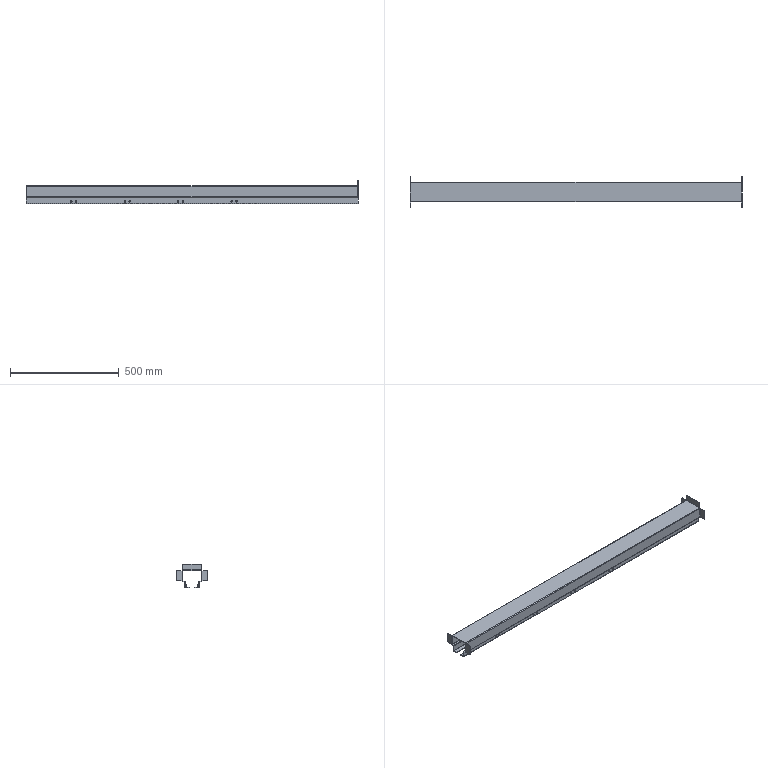Part | SolidWorks | features BaseBody 1 | 1 solid | 308 faces | box 1528 x 146 x 110.4 mm | volume 1185985 mm3 | plane 218 | cylinder 90 | commonest cylinder face diameters 6 x45 6.6 x32 1 x13